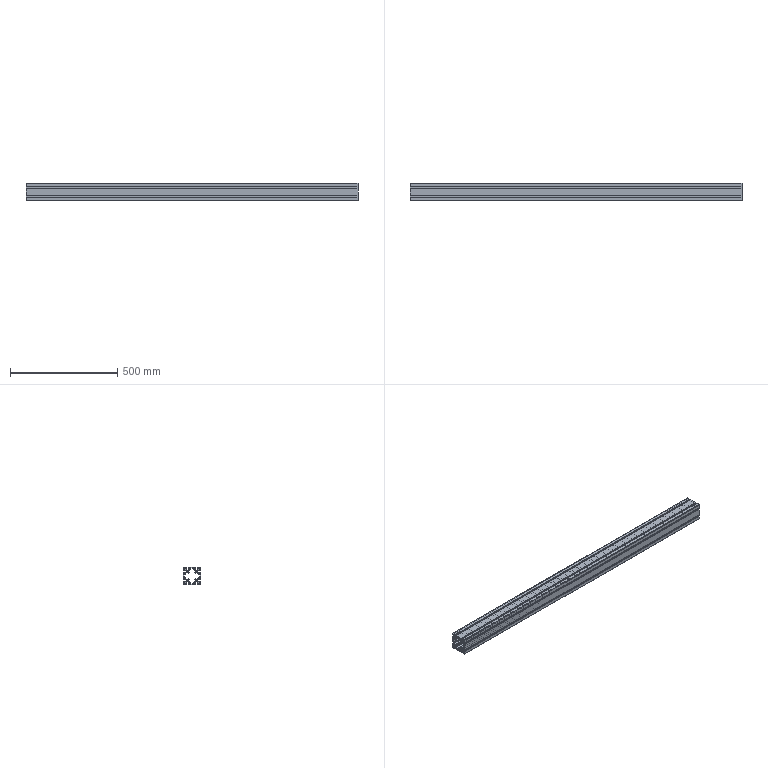Part | SolidWorks | features ICE 1, WeldMemberFeat 1, WeldmentFeature 1 | 1 solid | 174 faces | box 1550 x 80 x 80 mm | volume 3547982 mm3 | plane 146 | cylinder 28 | commonest cylinder face diameters 2 x8 6 x8 6.8 x8 3 x4